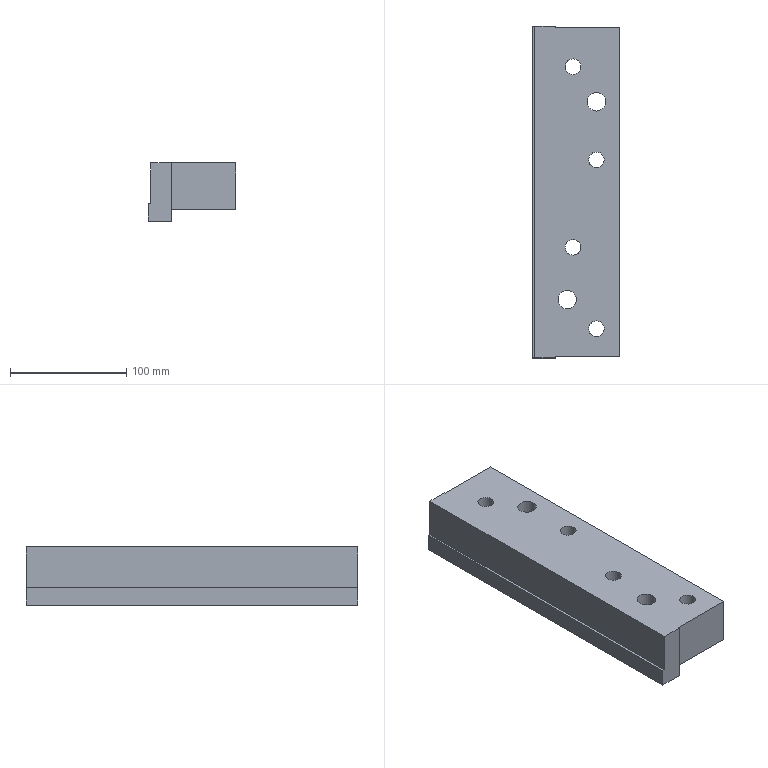Part | NX | features solid 2 | 1 solid | 26 faces | box 75 x 285 x 50 mm | volume 839332 mm3 | plane 16 | cylinder 10 | commonest cylinder face diameters 13.5 x4 19.5 x4 16 x2
STEP:
#1=CARTESIAN_POINT('',(1320.,-154.,3.));
#2=VERTEX_POINT('',#1);
#3=CARTESIAN_POINT('',(1320.,-154.,43.));
#4=VERTEX_POINT('',#3);
#5=CARTESIAN_POINT('',(1320.,-154.,-7.));
#6=DIRECTION('',(0.,0.,1.));
#7=VECTOR('',#6,1000.);
#8=LINE('',#5,#7);
#9=EDGE_CURVE('',#2,#4,#8,.T.);
#10=ORIENTED_EDGE('',*,*,#9,.F.);
#11=CARTESIAN_POINT('',(1320.,129.,3.));
#12=VERTEX_POINT('',#11);
#13=CARTESIAN_POINT('',(1320.,330.,3.));
#14=DIRECTION('',(0.,-1.,0.));
#15=VECTOR('',#14,1000.);
#16=LINE('',#13,#15);
#17=EDGE_CURVE('',#12,#2,#16,.T.);
#18=ORIENTED_EDGE('',*,*,#17,.F.);
#19=CARTESIAN_POINT('',(1320.,129.,43.));
#20=VERTEX_POINT('',#19);
#21=CARTESIAN_POINT('',(1320.,129.,-7.));
#22=DIRECTION('',(0.,0.,-1.));
#23=VECTOR('',#22,1000.);
#24=LINE('',#21,#23);
#25=EDGE_CURVE('',#20,#12,#24,.T.);
#26=ORIENTED_EDGE('',*,*,#25,.F.);
#27=CARTESIAN_POINT('',(1320.,330.,43.));
#28=DIRECTION('',(0.,-1.,0.));
#29=VECTOR('',#28,1000.);
#30=LINE('',#27,#29);
#31=EDGE_CURVE('',#20,#4,#30,.T.);
#32=ORIENTED_EDGE('',*,*,#31,.T.);
#33=EDGE_LOOP('',(#10,#18,#26,#32));
#34=FACE_BOUND('',#33,.T.);
#35=CARTESIAN_POINT('',(1320.,330.,-7.));
#36=DIRECTION('',(-1.,0.,0.));
#37=DIRECTION('',(0.,0.,1.));
#38=AXIS2_PLACEMENT_3D('',#35,#36,#37);
#39=PLANE('',#38);
#40=ADVANCED_FACE('',(#34),#39,.F.);
#41=CARTESIAN_POINT('',(1275.,-97.,43.));
#42=VERTEX_POINT('',#41);
#43=CARTESIAN_POINT('',(1275.,-105.,43.));
#44=DIRECTION('',(0.,0.,-1.));
#45=DIRECTION('',(0.,1.,0.));
#46=AXIS2_PLACEMENT_3D('',#43,#44,#45);
#47=CIRCLE('',#46,8.);
#48=EDGE_CURVE('',#42,#42,#47,.F.);
#49=ORIENTED_EDGE('',*,*,#48,.F.);
#50=EDGE_LOOP('',(#49));
#51=FACE_BOUND('',#50,.T.);
#52=CARTESIAN_POINT('',(1280.,101.75,43.));
#53=VERTEX_POINT('',#52);
#54=CARTESIAN_POINT('',(1280.,95.,43.));
#55=DIRECTION('',(0.,0.,-1.));
#56=DIRECTION('',(0.,1.,0.));
#57=AXIS2_PLACEMENT_3D('',#54,#55,#56);
#58=CIRCLE('',#57,6.75);
#59=EDGE_CURVE('',#53,#53,#58,.F.);
#60=ORIENTED_EDGE('',*,*,#59,.F.);
#61=EDGE_LOOP('',(#60));
#62=FACE_BOUND('',#61,.T.);
#63=CARTESIAN_POINT('',(1280.,-53.25,43.));
#64=VERTEX_POINT('',#63);
#65=CARTESIAN_POINT('',(1280.,-60.,43.));
#66=DIRECTION('',(0.,0.,-1.));
#67=DIRECTION('',(0.,1.,0.));
#68=AXIS2_PLACEMENT_3D('',#65,#66,#67);
#69=CIRCLE('',#68,6.75);
#70=EDGE_CURVE('',#64,#64,#69,.F.);
#71=ORIENTED_EDGE('',*,*,#70,.F.);
#72=EDGE_LOOP('',(#71));
#73=FACE_BOUND('',#72,.T.);
#74=CARTESIAN_POINT('',(1247.,-155.,43.));
#75=VERTEX_POINT('',#74);
#76=CARTESIAN_POINT('',(1265.,-155.,43.));
#77=VERTEX_POINT('',#76);
#78=CARTESIAN_POINT('',(1245.,-155.,43.));
#79=DIRECTION('',(1.,0.,0.));
#80=VECTOR('',#79,1000.);
#81=LINE('',#78,#80);
#82=EDGE_CURVE('',#75,#77,#81,.T.);
#83=ORIENTED_EDGE('',*,*,#82,.T.);
#84=CARTESIAN_POINT('',(1265.,-154.,43.));
#85=VERTEX_POINT('',#84);
#86=CARTESIAN_POINT('',(1265.,390.,43.));
#87=DIRECTION('',(0.,1.,0.));
#88=VECTOR('',#87,1000.);
#89=LINE('',#86,#88);
#90=EDGE_CURVE('',#77,#85,#89,.T.);
#91=ORIENTED_EDGE('',*,*,#90,.T.);
#92=CARTESIAN_POINT('',(1319.,-154.,43.));
#93=DIRECTION('',(1.,0.,0.));
#94=VECTOR('',#93,1000.);
#95=LINE('',#92,#94);
#96=EDGE_CURVE('',#85,#4,#95,.T.);
#97=ORIENTED_EDGE('',*,*,#96,.T.);
#98=ORIENTED_EDGE('',*,*,#31,.F.);
#99=CARTESIAN_POINT('',(1265.,129.,43.));
#100=VERTEX_POINT('',#99);
#101=CARTESIAN_POINT('',(1319.,129.,43.));
#102=DIRECTION('',(1.,0.,0.));
#103=VECTOR('',#102,1000.);
#104=LINE('',#101,#103);
#105=EDGE_CURVE('',#100,#20,#104,.T.);
#106=ORIENTED_EDGE('',*,*,#105,.F.);
#107=CARTESIAN_POINT('',(1265.,130.,43.));
#108=VERTEX_POINT('',#107);
#109=CARTESIAN_POINT('',(1265.,130.,43.));
#110=DIRECTION('',(0.,-1.,0.));
#111=VECTOR('',#110,1000.);
#112=LINE('',#109,#111);
#113=EDGE_CURVE('',#100,#108,#112,.F.);
#114=ORIENTED_EDGE('',*,*,#113,.T.);
#115=CARTESIAN_POINT('',(1247.,130.,43.));
#116=VERTEX_POINT('',#115);
#117=CARTESIAN_POINT('',(1245.,130.,43.));
#118=DIRECTION('',(1.,0.,0.));
#119=VECTOR('',#118,1000.);
#120=LINE('',#117,#119);
#121=EDGE_CURVE('',#116,#108,#120,.T.);
#122=ORIENTED_EDGE('',*,*,#121,.F.);
#123=CARTESIAN_POINT('',(1247.,390.,43.));
#124=DIRECTION('',(0.,1.,0.));
#125=VECTOR('',#124,1000.);
#126=LINE('',#123,#125);
#127=EDGE_CURVE('',#116,#75,#126,.F.);
#128=ORIENTED_EDGE('',*,*,#127,.T.);
#129=EDGE_LOOP('',(#83,#91,#97,#98,#106,#114,#122,#128));
#130=FACE_BOUND('',#129,.T.);
#131=CARTESIAN_POINT('',(1300.,-123.25,43.));
#132=VERTEX_POINT('',#131);
#133=CARTESIAN_POINT('',(1300.,-130.,43.));
#134=DIRECTION('',(0.,0.,-1.));
#135=DIRECTION('',(0.,1.,0.));
#136=AXIS2_PLACEMENT_3D('',#133,#134,#135);
#137=CIRCLE('',#136,6.75);
#138=EDGE_CURVE('',#132,#132,#137,.F.);
#139=ORIENTED_EDGE('',*,*,#138,.F.);
#140=EDGE_LOOP('',(#139));
#141=FACE_BOUND('',#140,.T.);
#142=CARTESIAN_POINT('',(1300.,21.75,43.));
#143=VERTEX_POINT('',#142);
#144=CARTESIAN_POINT('',(1300.,15.,43.));
#145=DIRECTION('',(0.,0.,-1.));
#146=DIRECTION('',(0.,1.,0.));
#147=AXIS2_PLACEMENT_3D('',#144,#145,#146);
#148=CIRCLE('',#147,6.75);
#149=EDGE_CURVE('',#143,#143,#148,.F.);
#150=ORIENTED_EDGE('',*,*,#149,.F.);
#151=EDGE_LOOP('',(#150));
#152=FACE_BOUND('',#151,.T.);
#153=CARTESIAN_POINT('',(1300.,73.,43.));
#154=VERTEX_POINT('',#153);
#155=CARTESIAN_POINT('',(1300.,65.,43.));
#156=DIRECTION('',(0.,0.,-1.));
#157=DIRECTION('',(0.,1.,0.));
#158=AXIS2_PLACEMENT_3D('',#155,#156,#157);
#159=CIRCLE('',#158,8.);
#160=EDGE_CURVE('',#154,#154,#159,.F.);
#161=ORIENTED_EDGE('',*,*,#160,.F.);
#162=EDGE_LOOP('',(#161));
#163=FACE_BOUND('',#162,.T.);
#164=CARTESIAN_POINT('',(1245.,390.,43.));
#165=DIRECTION('',(0.,0.,-1.));
#166=DIRECTION('',(0.,-1.,0.));
#167=AXIS2_PLACEMENT_3D('',#164,#165,#166);
#168=PLANE('',#167);
#169=ADVANCED_FACE('',(#51,#62,#73,#130,#141,#152,#163),#168,.F.);
#170=CARTESIAN_POINT('',(1265.,-154.,3.));
#171=VERTEX_POINT('',#170);
#172=CARTESIAN_POINT('',(1319.,-154.,3.));
#173=DIRECTION('',(1.,0.,0.));
#174=VECTOR('',#173,1000.);
#175=LINE('',#172,#174);
#176=EDGE_CURVE('',#171,#2,#175,.T.);
#177=ORIENTED_EDGE('',*,*,#176,.F.);
#178=CARTESIAN_POINT('',(1265.,129.,3.));
#179=VERTEX_POINT('',#178);
#180=CARTESIAN_POINT('',(1265.,130.,3.));
#181=DIRECTION('',(0.,-1.,0.));
#182=VECTOR('',#181,1000.);
#183=LINE('',#180,#182);
#184=EDGE_CURVE('',#179,#171,#183,.T.);
#185=ORIENTED_EDGE('',*,*,#184,.F.);
#186=CARTESIAN_POINT('',(1265.,129.,3.));
#187=DIRECTION('',(1.,0.,0.));
#188=VECTOR('',#187,1000.);
#189=LINE('',#186,#188);
#190=EDGE_CURVE('',#179,#12,#189,.T.);
#191=ORIENTED_EDGE('',*,*,#190,.T.);
#192=ORIENTED_EDGE('',*,*,#17,.T.);
#193=EDGE_LOOP('',(#177,#185,#191,#192));
#194=FACE_BOUND('',#193,.T.);
#195=CARTESIAN_POINT('',(1300.,24.75,3.));
#196=VERTEX_POINT('',#195);
#197=CARTESIAN_POINT('',(1300.,15.,3.));
#198=DIRECTION('',(0.,0.,-1.));
#199=DIRECTION('',(0.,1.,0.));
#200=AXIS2_PLACEMENT_3D('',#197,#198,#199);
#201=CIRCLE('',#200,9.75);
#202=EDGE_CURVE('',#196,#196,#201,.F.);
#203=ORIENTED_EDGE('',*,*,#202,.T.);
#204=EDGE_LOOP('',(#203));
#205=FACE_BOUND('',#204,.T.);
#206=CARTESIAN_POINT('',(1300.,-120.25,3.));
#207=VERTEX_POINT('',#206);
#208=CARTESIAN_POINT('',(1300.,-130.,3.));
#209=DIRECTION('',(0.,0.,-1.));
#210=DIRECTION('',(0.,1.,0.));
#211=AXIS2_PLACEMENT_3D('',#208,#209,#210);
#212=CIRCLE('',#211,9.75);
#213=EDGE_CURVE('',#207,#207,#212,.F.);
#214=ORIENTED_EDGE('',*,*,#213,.T.);
#215=EDGE_LOOP('',(#214));
#216=FACE_BOUND('',#215,.T.);
#217=CARTESIAN_POINT('',(1275.,-97.,3.));
#218=VERTEX_POINT('',#217);
#219=CARTESIAN_POINT('',(1275.,-105.,3.));
#220=DIRECTION('',(0.,0.,-1.));
#221=DIRECTION('',(0.,1.,0.));
#222=AXIS2_PLACEMENT_3D('',#219,#220,#221);
#223=CIRCLE('',#222,8.);
#224=EDGE_CURVE('',#218,#218,#223,.T.);
#225=ORIENTED_EDGE('',*,*,#224,.F.);
#226=EDGE_LOOP('',(#225));
#227=FACE_BOUND('',#226,.T.);
#228=CARTESIAN_POINT('',(1280.,-50.25,3.));
#229=VERTEX_POINT('',#228);
#230=CARTESIAN_POINT('',(1280.,-60.,3.));
#231=DIRECTION('',(0.,0.,-1.));
#232=DIRECTION('',(0.,1.,0.));
#233=AXIS2_PLACEMENT_3D('',#230,#231,#232);
#234=CIRCLE('',#233,9.75);
#235=EDGE_CURVE('',#229,#229,#234,.F.);
#236=ORIENTED_EDGE('',*,*,#235,.T.);
#237=EDGE_LOOP('',(#236));
#238=FACE_BOUND('',#237,.T.);
#239=CARTESIAN_POINT('',(1280.,104.75,3.));
#240=VERTEX_POINT('',#239);
#241=CARTESIAN_POINT('',(1280.,95.,3.));
#242=DIRECTION('',(0.,0.,-1.));
#243=DIRECTION('',(0.,1.,0.));
#244=AXIS2_PLACEMENT_3D('',#241,#242,#243);
#245=CIRCLE('',#244,9.75);
#246=EDGE_CURVE('',#240,#240,#245,.F.);
#247=ORIENTED_EDGE('',*,*,#246,.T.);
#248=EDGE_LOOP('',(#247));
#249=FACE_BOUND('',#248,.T.);
#250=CARTESIAN_POINT('',(1300.,73.,3.));
#251=VERTEX_POINT('',#250);
#252=CARTESIAN_POINT('',(1300.,65.,3.));
#253=DIRECTION('',(0.,0.,-1.));
#254=DIRECTION('',(0.,1.,0.));
#255=AXIS2_PLACEMENT_3D('',#252,#253,#254);
#256=CIRCLE('',#255,8.);
#257=EDGE_CURVE('',#251,#251,#256,.F.);
#258=ORIENTED_EDGE('',*,*,#257,.T.);
#259=EDGE_LOOP('',(#258));
#260=FACE_BOUND('',#259,.T.);
#261=CARTESIAN_POINT('',(1265.,130.,3.));
#262=DIRECTION('',(0.,0.,-1.));
#263=DIRECTION('',(0.,-1.,0.));
#264=AXIS2_PLACEMENT_3D('',#261,#262,#263);
#265=PLANE('',#264);
#266=ADVANCED_FACE('',(#194,#205,#216,#227,#238,#249,#260),#265,.T.);
#267=ORIENTED_EDGE('',*,*,#121,.T.);
#268=CARTESIAN_POINT('',(1265.,130.,-7.));
#269=VERTEX_POINT('',#268);
#270=CARTESIAN_POINT('',(1265.,130.,-7.));
#271=DIRECTION('',(0.,0.,1.));
#272=VECTOR('',#271,1000.);
#273=LINE('',#270,#272);
#274=EDGE_CURVE('',#269,#108,#273,.T.);
#275=ORIENTED_EDGE('',*,*,#274,.F.);
#276=CARTESIAN_POINT('',(1245.,130.,-7.));
#277=VERTEX_POINT('',#276);
#278=CARTESIAN_POINT('',(1245.,130.,-7.));
#279=DIRECTION('',(1.,0.,0.));
#280=VECTOR('',#279,1000.);
#281=LINE('',#278,#280);
#282=EDGE_CURVE('',#269,#277,#281,.F.);
#283=ORIENTED_EDGE('',*,*,#282,.T.);
#284=CARTESIAN_POINT('',(1245.,130.,8.));
#285=VERTEX_POINT('',#284);
#286=CARTESIAN_POINT('',(1245.,130.,-7.));
#287=DIRECTION('',(0.,0.,-1.));
#288=VECTOR('',#287,1000.);
#289=LINE('',#286,#288);
#290=EDGE_CURVE('',#285,#277,#289,.T.);
#291=ORIENTED_EDGE('',*,*,#290,.F.);
#292=CARTESIAN_POINT('',(1247.,130.,8.));
#293=VERTEX_POINT('',#292);
#294=CARTESIAN_POINT('',(1245.,130.,8.));
#295=DIRECTION('',(-1.,0.,0.));
#296=VECTOR('',#295,1000.);
#297=LINE('',#294,#296);
#298=EDGE_CURVE('',#285,#293,#297,.F.);
#299=ORIENTED_EDGE('',*,*,#298,.T.);
#300=CARTESIAN_POINT('',(1247.,130.,43.));
#301=DIRECTION('',(0.,0.,1.));
#302=VECTOR('',#301,1000.);
#303=LINE('',#300,#302);
#304=EDGE_CURVE('',#293,#116,#303,.T.);
#305=ORIENTED_EDGE('',*,*,#304,.T.);
#306=EDGE_LOOP('',(#267,#275,#283,#291,#299,#305));
#307=FACE_BOUND('',#306,.T.);
#308=CARTESIAN_POINT('',(1305.,130.,-7.));
#309=DIRECTION('',(0.,1.,0.));
#310=DIRECTION('',(0.,0.,1.));
#311=AXIS2_PLACEMENT_3D('',#308,#309,#310);
#312=PLANE('',#311);
#313=ADVANCED_FACE('',(#307),#312,.T.);
#314=CARTESIAN_POINT('',(1265.,-155.,-7.));
#315=VERTEX_POINT('',#314);
#316=CARTESIAN_POINT('',(1265.,-155.,-7.));
#317=DIRECTION('',(0.,0.,1.));
#318=VECTOR('',#317,1000.);
#319=LINE('',#316,#318);
#320=EDGE_CURVE('',#315,#77,#319,.T.);
#321=ORIENTED_EDGE('',*,*,#320,.T.);
#322=ORIENTED_EDGE('',*,*,#82,.F.);
#323=CARTESIAN_POINT('',(1247.,-155.,8.));
#324=VERTEX_POINT('',#323);
#325=CARTESIAN_POINT('',(1247.,-155.,43.));
#326=DIRECTION('',(0.,0.,1.));
#327=VECTOR('',#326,1000.);
#328=LINE('',#325,#327);
#329=EDGE_CURVE('',#324,#75,#328,.T.);
#330=ORIENTED_EDGE('',*,*,#329,.F.);
#331=CARTESIAN_POINT('',(1245.,-155.,8.));
#332=VERTEX_POINT('',#331);
#333=CARTESIAN_POINT('',(1245.,-155.,8.));
#334=DIRECTION('',(-1.,0.,0.));
#335=VECTOR('',#334,1000.);
#336=LINE('',#333,#335);
#337=EDGE_CURVE('',#332,#324,#336,.F.);
#338=ORIENTED_EDGE('',*,*,#337,.F.);
#339=CARTESIAN_POINT('',(1245.,-155.,-7.));
#340=VERTEX_POINT('',#339);
#341=CARTESIAN_POINT('',(1245.,-155.,-7.));
#342=DIRECTION('',(0.,0.,-1.));
#343=VECTOR('',#342,1000.);
#344=LINE('',#341,#343);
#345=EDGE_CURVE('',#332,#340,#344,.T.);
#346=ORIENTED_EDGE('',*,*,#345,.T.);
#347=CARTESIAN_POINT('',(1245.,-155.,-7.));
#348=DIRECTION('',(1.,0.,0.));
#349=VECTOR('',#348,1000.);
#350=LINE('',#347,#349);
#351=EDGE_CURVE('',#315,#340,#350,.F.);
#352=ORIENTED_EDGE('',*,*,#351,.F.);
#353=EDGE_LOOP('',(#321,#322,#330,#338,#346,#352));
#354=FACE_BOUND('',#353,.T.);
#355=CARTESIAN_POINT('',(1305.,-155.,-7.));
#356=DIRECTION('',(0.,1.,0.));
#357=DIRECTION('',(0.,0.,1.));
#358=AXIS2_PLACEMENT_3D('',#355,#356,#357);
#359=PLANE('',#358);
#360=ADVANCED_FACE('',(#354),#359,.F.);
#361=CARTESIAN_POINT('',(1280.,85.25,18.));
#362=VERTEX_POINT('',#361);
#363=CARTESIAN_POINT('',(1280.,95.,18.));
#364=DIRECTION('',(0.,0.,1.));
#365=DIRECTION('',(0.,-1.,0.));
#366=AXIS2_PLACEMENT_3D('',#363,#364,#365);
#367=CIRCLE('',#366,9.75);
#368=EDGE_CURVE('',#362,#362,#367,.T.);
#369=ORIENTED_EDGE('',*,*,#368,.T.);
#370=EDGE_LOOP('',(#369));
#371=FACE_BOUND('',#370,.T.);
#372=ORIENTED_EDGE('',*,*,#246,.F.);
#373=EDGE_LOOP('',(#372));
#374=FACE_BOUND('',#373,.T.);
#375=CARTESIAN_POINT('',(1280.,95.,-82.));
#376=DIRECTION('',(0.,0.,1.));
#377=DIRECTION('',(1.,0.,0.));
#378=AXIS2_PLACEMENT_3D('',#375,#376,#377);
#379=CYLINDRICAL_SURFACE('',#378,9.75);
#380=ADVANCED_FACE('',(#371,#374),#379,.F.);
#381=CARTESIAN_POINT('',(1300.,5.25,18.));
#382=VERTEX_POINT('',#381);
#383=CARTESIAN_POINT('',(1300.,15.,18.));
#384=DIRECTION('',(0.,0.,1.));
#385=DIRECTION('',(0.,-1.,0.));
#386=AXIS2_PLACEMENT_3D('',#383,#384,#385);
#387=CIRCLE('',#386,9.75);
#388=EDGE_CURVE('',#382,#382,#387,.T.);
#389=ORIENTED_EDGE('',*,*,#388,.T.);
#390=EDGE_LOOP('',(#389));
#391=FACE_BOUND('',#390,.T.);
#392=ORIENTED_EDGE('',*,*,#202,.F.);
#393=EDGE_LOOP('',(#392));
#394=FACE_BOUND('',#393,.T.);
#395=CARTESIAN_POINT('',(1300.,15.,-82.));
#396=DIRECTION('',(0.,0.,1.));
#397=DIRECTION('',(1.,0.,0.));
#398=AXIS2_PLACEMENT_3D('',#395,#396,#397);
#399=CYLINDRICAL_SURFACE('',#398,9.75);
#400=ADVANCED_FACE('',(#391,#394),#399,.F.);
#401=CARTESIAN_POINT('',(1280.,-69.75,18.));
#402=VERTEX_POINT('',#401);
#403=CARTESIAN_POINT('',(1280.,-60.,18.));
#404=DIRECTION('',(0.,0.,1.));
#405=DIRECTION('',(0.,-1.,0.));
#406=AXIS2_PLACEMENT_3D('',#403,#404,#405);
#407=CIRCLE('',#406,9.75);
#408=EDGE_CURVE('',#402,#402,#407,.T.);
#409=ORIENTED_EDGE('',*,*,#408,.T.);
#410=EDGE_LOOP('',(#409));
#411=FACE_BOUND('',#410,.T.);
#412=ORIENTED_EDGE('',*,*,#235,.F.);
#413=EDGE_LOOP('',(#412));
#414=FACE_BOUND('',#413,.T.);
#415=CARTESIAN_POINT('',(1280.,-60.,-82.));
#416=DIRECTION('',(0.,0.,1.));
#417=DIRECTION('',(1.,0.,0.));
#418=AXIS2_PLACEMENT_3D('',#415,#416,#417);
#419=CYLINDRICAL_SURFACE('',#418,9.75);
#420=ADVANCED_FACE('',(#411,#414),#419,.F.);
#421=CARTESIAN_POINT('',(1300.,-139.75,18.));
#422=VERTEX_POINT('',#421);
#423=CARTESIAN_POINT('',(1300.,-130.,18.));
#424=DIRECTION('',(0.,0.,1.));
#425=DIRECTION('',(0.,-1.,0.));
#426=AXIS2_PLACEMENT_3D('',#423,#424,#425);
#427=CIRCLE('',#426,9.75);
#428=EDGE_CURVE('',#422,#422,#427,.T.);
#429=ORIENTED_EDGE('',*,*,#428,.T.);
#430=EDGE_LOOP('',(#429));
#431=FACE_BOUND('',#430,.T.);
#432=ORIENTED_EDGE('',*,*,#213,.F.);
#433=EDGE_LOOP('',(#432));
#434=FACE_BOUND('',#433,.T.);
#435=CARTESIAN_POINT('',(1300.,-130.,-82.));
#436=DIRECTION('',(0.,0.,1.));
#437=DIRECTION('',(1.,0.,0.));
#438=AXIS2_PLACEMENT_3D('',#435,#436,#437);
#439=CYLINDRICAL_SURFACE('',#438,9.75);
#440=ADVANCED_FACE('',(#431,#434),#439,.F.);
#441=ORIENTED_EDGE('',*,*,#48,.T.);
#442=EDGE_LOOP('',(#441));
#443=FACE_BOUND('',#442,.T.);
#444=ORIENTED_EDGE('',*,*,#224,.T.);
#445=EDGE_LOOP('',(#444));
#446=FACE_BOUND('',#445,.T.);
#447=CARTESIAN_POINT('',(1275.,-105.,93.));
#448=DIRECTION('',(0.,0.,-1.));
#449=DIRECTION('',(-1.,0.,0.));
#450=AXIS2_PLACEMENT_3D('',#447,#448,#449);
#451=CYLINDRICAL_SURFACE('',#450,8.);
#452=ADVANCED_FACE('',(#443,#446),#451,.F.);
#453=ORIENTED_EDGE('',*,*,#282,.F.);
#454=CARTESIAN_POINT('',(1265.,330.,-7.));
#455=DIRECTION('',(0.,1.,0.));
#456=VECTOR('',#455,1000.);
#457=LINE('',#454,#456);
#458=EDGE_CURVE('',#269,#315,#457,.F.);
#459=ORIENTED_EDGE('',*,*,#458,.T.);
#460=ORIENTED_EDGE('',*,*,#351,.T.);
#461=CARTESIAN_POINT('',(1245.,330.,-7.));
#462=DIRECTION('',(0.,1.,0.));
#463=VECTOR('',#462,1000.);
#464=LINE('',#461,#463);
#465=EDGE_CURVE('',#277,#340,#464,.F.);
#466=ORIENTED_EDGE('',*,*,#465,.F.);
#467=EDGE_LOOP('',(#453,#459,#460,#466));
#468=FACE_BOUND('',#467,.T.);
#469=CARTESIAN_POINT('',(1245.,330.,-7.));
#470=DIRECTION('',(0.,0.,-1.));
#471=DIRECTION('',(0.,-1.,0.));
#472=AXIS2_PLACEMENT_3D('',#469,#470,#471);
#473=PLANE('',#472);
#474=ADVANCED_FACE('',(#468),#473,.T.);
#475=CARTESIAN_POINT('',(1247.,390.,8.));
#476=DIRECTION('',(0.,1.,0.));
#477=VECTOR('',#476,1000.);
#478=LINE('',#475,#477);
#479=EDGE_CURVE('',#293,#324,#478,.F.);
#480=ORIENTED_EDGE('',*,*,#479,.T.);
#481=ORIENTED_EDGE('',*,*,#329,.T.);
#482=ORIENTED_EDGE('',*,*,#127,.F.);
#483=ORIENTED_EDGE('',*,*,#304,.F.);
#484=EDGE_LOOP('',(#480,#481,#482,#483));
#485=FACE_BOUND('',#484,.T.);
#486=CARTESIAN_POINT('',(1247.,390.,43.));
#487=DIRECTION('',(1.,0.,0.));
#488=DIRECTION('',(0.,0.,-1.));
#489=AXIS2_PLACEMENT_3D('',#486,#487,#488);
#490=PLANE('',#489);
#491=ADVANCED_FACE('',(#485),#490,.F.);
#492=CARTESIAN_POINT('',(1245.,390.,8.));
#493=DIRECTION('',(0.,-1.,0.));
#494=VECTOR('',#493,1000.);
#495=LINE('',#492,#494);
#496=EDGE_CURVE('',#285,#332,#495,.T.);
#497=ORIENTED_EDGE('',*,*,#496,.T.);
#498=ORIENTED_EDGE('',*,*,#337,.T.);
#499=ORIENTED_EDGE('',*,*,#479,.F.);
#500=ORIENTED_EDGE('',*,*,#298,.F.);
#501=EDGE_LOOP('',(#497,#498,#499,#500));
#502=FACE_BOUND('',#501,.T.);
#503=CARTESIAN_POINT('',(1245.,390.,8.));
#504=DIRECTION('',(0.,0.,1.));
#505=DIRECTION('',(0.,-1.,0.));
#506=AXIS2_PLACEMENT_3D('',#503,#504,#505);
#507=PLANE('',#506);
#508=ADVANCED_FACE('',(#502),#507,.T.);
#509=ORIENTED_EDGE('',*,*,#345,.F.);
#510=ORIENTED_EDGE('',*,*,#496,.F.);
#511=ORIENTED_EDGE('',*,*,#290,.T.);
#512=ORIENTED_EDGE('',*,*,#465,.T.);
#513=EDGE_LOOP('',(#509,#510,#511,#512));
#514=FACE_BOUND('',#513,.T.);
#515=CARTESIAN_POINT('',(1245.,390.,-7.));
#516=DIRECTION('',(-1.,0.,0.));
#517=DIRECTION('',(0.,0.,1.));
#518=AXIS2_PLACEMENT_3D('',#515,#516,#517);
#519=PLANE('',#518);
#520=ADVANCED_FACE('',(#514),#519,.T.);
#521=CARTESIAN_POINT('',(1306.75,-130.,18.));
#522=VERTEX_POINT('',#521);
#523=CARTESIAN_POINT('',(1300.,-130.,18.));
#524=DIRECTION('',(0.,0.,1.));
#525=DIRECTION('',(1.,0.,0.));
#526=AXIS2_PLACEMENT_3D('',#523,#524,#525);
#527=CIRCLE('',#526,6.75);
#528=EDGE_CURVE('',#522,#522,#527,.T.);
#529=ORIENTED_EDGE('',*,*,#528,.F.);
#530=EDGE_LOOP('',(#529));
#531=FACE_BOUND('',#530,.T.);
#532=ORIENTED_EDGE('',*,*,#138,.T.);
#533=EDGE_LOOP('',(#532));
#534=FACE_BOUND('',#533,.T.);
#535=CARTESIAN_POINT('',(1300.,-130.,118.));
#536=DIRECTION('',(0.,0.,-1.));
#537=DIRECTION('',(-1.,0.,0.));
#538=AXIS2_PLACEMENT_3D('',#535,#536,#537);
#539=CYLINDRICAL_SURFACE('',#538,6.75);
#540=ADVANCED_FACE('',(#531,#534),#539,.F.);
#541=CARTESIAN_POINT('',(1286.75,-60.,18.));
#542=VERTEX_POINT('',#541);
#543=CARTESIAN_POINT('',(1280.,-60.,18.));
#544=DIRECTION('',(0.,0.,1.));
#545=DIRECTION('',(1.,0.,0.));
#546=AXIS2_PLACEMENT_3D('',#543,#544,#545);
#547=CIRCLE('',#546,6.75);
#548=EDGE_CURVE('',#542,#542,#547,.T.);
#549=ORIENTED_EDGE('',*,*,#548,.F.);
#550=EDGE_LOOP('',(#549));
#551=FACE_BOUND('',#550,.T.);
#552=ORIENTED_EDGE('',*,*,#70,.T.);
#553=EDGE_LOOP('',(#552));
#554=FACE_BOUND('',#553,.T.);
#555=CARTESIAN_POINT('',(1280.,-60.,118.));
#556=DIRECTION('',(0.,0.,-1.));
#557=DIRECTION('',(-1.,0.,0.));
#558=AXIS2_PLACEMENT_3D('',#555,#556,#557);
#559=CYLINDRICAL_SURFACE('',#558,6.75);
#560=ADVANCED_FACE('',(#551,#554),#559,.F.);
#561=CARTESIAN_POINT('',(1306.75,15.,18.));
#562=VERTEX_POINT('',#561);
#563=CARTESIAN_POINT('',(1300.,15.,18.));
#564=DIRECTION('',(0.,0.,1.));
#565=DIRECTION('',(1.,0.,0.));
#566=AXIS2_PLACEMENT_3D('',#563,#564,#565);
#567=CIRCLE('',#566,6.75);
#568=EDGE_CURVE('',#562,#562,#567,.T.);
#569=ORIENTED_EDGE('',*,*,#568,.F.);
#570=EDGE_LOOP('',(#569));
#571=FACE_BOUND('',#570,.T.);
#572=ORIENTED_EDGE('',*,*,#149,.T.);
#573=EDGE_LOOP('',(#572));
#574=FACE_BOUND('',#573,.T.);
#575=CARTESIAN_POINT('',(1300.,15.,118.));
#576=DIRECTION('',(0.,0.,-1.));
#577=DIRECTION('',(-1.,0.,0.));
#578=AXIS2_PLACEMENT_3D('',#575,#576,#577);
#579=CYLINDRICAL_SURFACE('',#578,6.75);
#580=ADVANCED_FACE('',(#571,#574),#579,.F.);
#581=CARTESIAN_POINT('',(1286.75,95.,18.));
#582=VERTEX_POINT('',#581);
#583=CARTESIAN_POINT('',(1280.,95.,18.));
#584=DIRECTION('',(0.,0.,1.));
#585=DIRECTION('',(1.,0.,0.));
#586=AXIS2_PLACEMENT_3D('',#583,#584,#585);
#587=CIRCLE('',#586,6.75);
#588=EDGE_CURVE('',#582,#582,#587,.T.);
#589=ORIENTED_EDGE('',*,*,#588,.F.);
#590=EDGE_LOOP('',(#589));
#591=FACE_BOUND('',#590,.T.);
#592=ORIENTED_EDGE('',*,*,#59,.T.);
#593=EDGE_LOOP('',(#592));
#594=FACE_BOUND('',#593,.T.);
#595=CARTESIAN_POINT('',(1280.,95.,118.));
#596=DIRECTION('',(0.,0.,-1.));
#597=DIRECTION('',(-1.,0.,0.));
#598=AXIS2_PLACEMENT_3D('',#595,#596,#597);
#599=CYLINDRICAL_SURFACE('',#598,6.75);
#600=ADVANCED_FACE('',(#591,#594),#599,.F.);
#601=ORIENTED_EDGE('',*,*,#588,.T.);
#602=EDGE_LOOP('',(#601));
#603=FACE_BOUND('',#602,.T.);
#604=ORIENTED_EDGE('',*,*,#368,.F.);
#605=EDGE_LOOP('',(#604));
#606=FACE_BOUND('',#605,.T.);
#607=CARTESIAN_POINT('',(1280.,95.,18.));
#608=DIRECTION('',(0.,0.,1.));
#609=DIRECTION('',(1.,0.,0.));
#610=AXIS2_PLACEMENT_3D('',#607,#608,#609);
#611=PLANE('',#610);
#612=ADVANCED_FACE('',(#603,#606),#611,.F.);
#613=ORIENTED_EDGE('',*,*,#568,.T.);
#614=EDGE_LOOP('',(#613));
#615=FACE_BOUND('',#614,.T.);
#616=ORIENTED_EDGE('',*,*,#388,.F.);
#617=EDGE_LOOP('',(#616));
#618=FACE_BOUND('',#617,.T.);
#619=CARTESIAN_POINT('',(1300.,15.,18.));
#620=DIRECTION('',(0.,0.,1.));
#621=DIRECTION('',(1.,0.,0.));
#622=AXIS2_PLACEMENT_3D('',#619,#620,#621);
#623=PLANE('',#622);
#624=ADVANCED_FACE('',(#615,#618),#623,.F.);
#625=ORIENTED_EDGE('',*,*,#548,.T.);
#626=EDGE_LOOP('',(#625));
#627=FACE_BOUND('',#626,.T.);
#628=ORIENTED_EDGE('',*,*,#408,.F.);
#629=EDGE_LOOP('',(#628));
#630=FACE_BOUND('',#629,.T.);
#631=CARTESIAN_POINT('',(1280.,-60.,18.));
#632=DIRECTION('',(0.,0.,1.));
#633=DIRECTION('',(1.,0.,0.));
#634=AXIS2_PLACEMENT_3D('',#631,#632,#633);
#635=PLANE('',#634);
#636=ADVANCED_FACE('',(#627,#630),#635,.F.);
#637=ORIENTED_EDGE('',*,*,#528,.T.);
#638=EDGE_LOOP('',(#637));
#639=FACE_BOUND('',#638,.T.);
#640=ORIENTED_EDGE('',*,*,#428,.F.);
#641=EDGE_LOOP('',(#640));
#642=FACE_BOUND('',#641,.T.);
#643=CARTESIAN_POINT('',(1300.,-130.,18.));
#644=DIRECTION('',(0.,0.,1.));
#645=DIRECTION('',(1.,0.,0.));
#646=AXIS2_PLACEMENT_3D('',#643,#644,#645);
#647=PLANE('',#646);
#648=ADVANCED_FACE('',(#639,#642),#647,.F.);
#649=ORIENTED_EDGE('',*,*,#184,.T.);
#650=CARTESIAN_POINT('',(1265.,-154.,-7.));
#651=DIRECTION('',(0.,0.,1.));
#652=VECTOR('',#651,1000.);
#653=LINE('',#650,#652);
#654=EDGE_CURVE('',#85,#171,#653,.F.);
#655=ORIENTED_EDGE('',*,*,#654,.F.);
#656=ORIENTED_EDGE('',*,*,#90,.F.);
#657=ORIENTED_EDGE('',*,*,#320,.F.);
#658=ORIENTED_EDGE('',*,*,#458,.F.);
#659=ORIENTED_EDGE('',*,*,#274,.T.);
#660=ORIENTED_EDGE('',*,*,#113,.F.);
#661=CARTESIAN_POINT('',(1265.,129.,-7.));
#662=DIRECTION('',(0.,0.,-1.));
#663=VECTOR('',#662,1000.);
#664=LINE('',#661,#663);
#665=EDGE_CURVE('',#179,#100,#664,.F.);
#666=ORIENTED_EDGE('',*,*,#665,.F.);
#667=EDGE_LOOP('',(#649,#655,#656,#657,#658,#659,#660,#666));
#668=FACE_BOUND('',#667,.T.);
#669=CARTESIAN_POINT('',(1265.,130.,-7.));
#670=DIRECTION('',(-1.,0.,0.));
#671=DIRECTION('',(0.,0.,1.));
#672=AXIS2_PLACEMENT_3D('',#669,#670,#671);
#673=PLANE('',#672);
#674=ADVANCED_FACE('',(#668),#673,.F.);
#675=ORIENTED_EDGE('',*,*,#257,.F.);
#676=EDGE_LOOP('',(#675));
#677=FACE_BOUND('',#676,.T.);
#678=ORIENTED_EDGE('',*,*,#160,.T.);
#679=EDGE_LOOP('',(#678));
#680=FACE_BOUND('',#679,.T.);
#681=CARTESIAN_POINT('',(1300.,65.,103.));
#682=DIRECTION('',(0.,0.,-1.));
#683=DIRECTION('',(-1.,0.,0.));
#684=AXIS2_PLACEMENT_3D('',#681,#682,#683);
#685=CYLINDRICAL_SURFACE('',#684,8.);
#686=ADVANCED_FACE('',(#677,#680),#685,.F.);
#687=ORIENTED_EDGE('',*,*,#665,.T.);
#688=ORIENTED_EDGE('',*,*,#105,.T.);
#689=ORIENTED_EDGE('',*,*,#25,.T.);
#690=ORIENTED_EDGE('',*,*,#190,.F.);
#691=EDGE_LOOP('',(#687,#688,#689,#690));
#692=FACE_BOUND('',#691,.T.);
#693=CARTESIAN_POINT('',(1319.,129.,-7.));
#694=DIRECTION('',(0.,1.,0.));
#695=DIRECTION('',(0.,0.,1.));
#696=AXIS2_PLACEMENT_3D('',#693,#694,#695);
#697=PLANE('',#696);
#698=ADVANCED_FACE('',(#692),#697,.T.);
#699=ORIENTED_EDGE('',*,*,#9,.T.);
#700=ORIENTED_EDGE('',*,*,#96,.F.);
#701=ORIENTED_EDGE('',*,*,#654,.T.);
#702=ORIENTED_EDGE('',*,*,#176,.T.);
#703=EDGE_LOOP('',(#699,#700,#701,#702));
#704=FACE_BOUND('',#703,.T.);
#705=CARTESIAN_POINT('',(1319.,-154.,43.));
#706=DIRECTION('',(0.,-1.,0.));
#707=DIRECTION('',(0.,0.,-1.));
#708=AXIS2_PLACEMENT_3D('',#705,#706,#707);
#709=PLANE('',#708);
#710=ADVANCED_FACE('',(#704),#709,.T.);
#711=CLOSED_SHELL('',(#40,#169,#266,#313,#360,#380,#400,#420,#440,#452,#474,#491,#508,#520,#540,#560,#580,#600,#612,#624,#636,#648,#674,#686,#698,#710));
#712=MANIFOLD_SOLID_BREP('',#711);
#713=(LENGTH_UNIT()NAMED_UNIT(*)SI_UNIT(.MILLI.,.METRE.));
#714=UNCERTAINTY_MEASURE_WITH_UNIT(LENGTH_MEASURE(0.00001),#713,'','');
#715=(NAMED_UNIT(*)PLANE_ANGLE_UNIT()SI_UNIT($,.RADIAN.));
#716=(NAMED_UNIT(*)SI_UNIT($,.STERADIAN.)SOLID_ANGLE_UNIT());
#717=(GEOMETRIC_REPRESENTATION_CONTEXT(3)GLOBAL_UNCERTAINTY_ASSIGNED_CONTEXT((#714))GLOBAL_UNIT_ASSIGNED_CONTEXT((#713,#715,#716))REPRESENTATION_CONTEXT('',''));
#718=ADVANCED_BREP_SHAPE_REPRESENTATION('',(#712),#717);